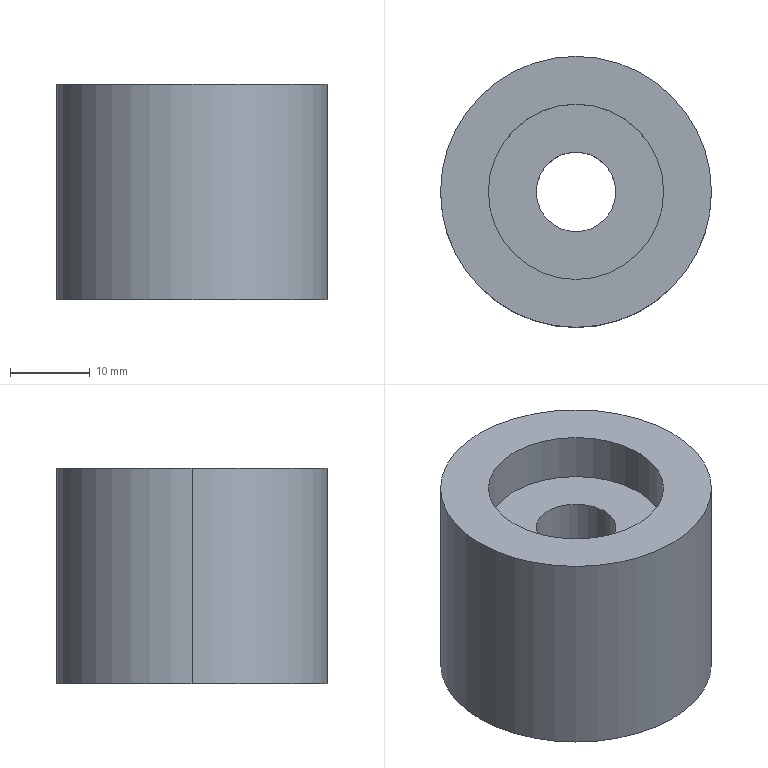Part | STEP file | Driven pulley shaft QY-1-34 | 1 solid | 12 faces | box 34 x 34 x 27 mm | volume 18774 mm3 | cylinder 8 | plane 4 | commonest cylinder face diameters 22 x4 10 x2 34 x2
STEP:
#1=CARTESIAN_POINT('',(0.,0.,0.));
#2=DIRECTION('',(0.,0.,1.));
#3=DIRECTION('',(1.,0.,0.));
#4=AXIS2_PLACEMENT_3D('',#1,#2,#3);
#5=CARTESIAN_POINT('',(-11.,0.,6.));
#6=VERTEX_POINT('',#5);
#7=CARTESIAN_POINT('',(-11.,0.,0.));
#8=VERTEX_POINT('',#7);
#9=CARTESIAN_POINT('',(-11.,0.,6.));
#10=DIRECTION('',(0.,0.,-1.));
#11=VECTOR('',#10,1.);
#12=LINE('',#9,#11);
#13=CARTESIAN_POINT('',(0.,0.,6.));
#14=DIRECTION('',(0.,0.,-1.));
#15=DIRECTION('',(-1.,0.,0.));
#16=AXIS2_PLACEMENT_3D('',#13,#14,#15);
#17=CYLINDRICAL_SURFACE('',#16,11.);
#18=CARTESIAN_POINT('',(6.283,0.));
#19=DIRECTION('',(0.,1.));
#20=VECTOR('',#19,1.);
#21=LINE('',#18,#20);
#22=(GEOMETRIC_REPRESENTATION_CONTEXT(2)PARAMETRIC_REPRESENTATION_CONTEXT()REPRESENTATION_CONTEXT('',''));
#23=DEFINITIONAL_REPRESENTATION('',(#21),#22);
#24=PCURVE('',#17,#23);
#25=CARTESIAN_POINT('',(0.,0.,6.));
#26=DIRECTION('',(0.,0.,-1.));
#27=DIRECTION('',(-1.,0.,0.));
#28=AXIS2_PLACEMENT_3D('',#25,#26,#27);
#29=CYLINDRICAL_SURFACE('',#28,11.);
#30=CARTESIAN_POINT('',(0.,0.));
#31=DIRECTION('',(0.,1.));
#32=VECTOR('',#31,1.);
#33=LINE('',#30,#32);
#34=(GEOMETRIC_REPRESENTATION_CONTEXT(2)PARAMETRIC_REPRESENTATION_CONTEXT()REPRESENTATION_CONTEXT('',''));
#35=DEFINITIONAL_REPRESENTATION('',(#33),#34);
#36=PCURVE('',#29,#35);
#37=SURFACE_CURVE('',#12,(#24,#36),.PCURVE_S1.);
#38=EDGE_CURVE('',#6,#8,#37,.T.);
#39=ORIENTED_EDGE('',*,*,#38,.T.);
#40=CARTESIAN_POINT('',(11.,0.,0.));
#41=VERTEX_POINT('',#40);
#42=CARTESIAN_POINT('',(0.,0.,0.));
#43=DIRECTION('',(0.,0.,-1.));
#44=DIRECTION('',(-1.,0.,0.));
#45=AXIS2_PLACEMENT_3D('',#42,#43,#44);
#46=CIRCLE('',#45,11.);
#47=CARTESIAN_POINT('',(0.,6.));
#48=DIRECTION('',(1.,0.));
#49=VECTOR('',#48,1.);
#50=LINE('',#47,#49);
#51=(GEOMETRIC_REPRESENTATION_CONTEXT(2)PARAMETRIC_REPRESENTATION_CONTEXT()REPRESENTATION_CONTEXT('',''));
#52=DEFINITIONAL_REPRESENTATION('',(#50),#51);
#53=PCURVE('',#17,#52);
#54=CARTESIAN_POINT('',(0.,0.,0.));
#55=DIRECTION('',(0.,0.,1.));
#56=DIRECTION('',(1.,0.,0.));
#57=AXIS2_PLACEMENT_3D('',#54,#55,#56);
#58=PLANE('',#57);
#59=CARTESIAN_POINT('',(-11.,0.));
#60=CARTESIAN_POINT('',(-11.,19.053));
#61=CARTESIAN_POINT('',(5.5,9.526));
#62=CARTESIAN_POINT('',(22.,0.));
#63=CARTESIAN_POINT('',(5.5,-9.526));
#64=CARTESIAN_POINT('',(-11.,-19.053));
#65=CARTESIAN_POINT('',(-11.,0.));
#66=(BOUNDED_CURVE()B_SPLINE_CURVE(2,(#59,#60,#61,#62,#63,#64,#65),.UNSPECIFIED.,.T.,.F.)B_SPLINE_CURVE_WITH_KNOTS((1,2,2,2,2,1),(-2.094,0.,2.094,4.189,6.283,8.378),.UNSPECIFIED.)CURVE()GEOMETRIC_REPRESENTATION_ITEM()RATIONAL_B_SPLINE_CURVE((1.,0.5,1.,0.5,1.,0.5,1.))REPRESENTATION_ITEM(''));
#67=(GEOMETRIC_REPRESENTATION_CONTEXT(2)PARAMETRIC_REPRESENTATION_CONTEXT()REPRESENTATION_CONTEXT('',''));
#68=DEFINITIONAL_REPRESENTATION('',(#66),#67);
#69=PCURVE('',#58,#68);
#70=SURFACE_CURVE('',#46,(#53,#69),.PCURVE_S1.);
#71=EDGE_CURVE('',#41,#8,#70,.T.);
#72=ORIENTED_EDGE('',*,*,#71,.F.);
#73=CARTESIAN_POINT('',(11.,0.,6.));
#74=VERTEX_POINT('',#73);
#75=CARTESIAN_POINT('',(11.,0.,6.));
#76=DIRECTION('',(0.,0.,-1.));
#77=VECTOR('',#76,1.);
#78=LINE('',#75,#77);
#79=CARTESIAN_POINT('',(3.142,0.));
#80=DIRECTION('',(0.,1.));
#81=VECTOR('',#80,1.);
#82=LINE('',#79,#81);
#83=(GEOMETRIC_REPRESENTATION_CONTEXT(2)PARAMETRIC_REPRESENTATION_CONTEXT()REPRESENTATION_CONTEXT('',''));
#84=DEFINITIONAL_REPRESENTATION('',(#82),#83);
#85=PCURVE('',#17,#84);
#86=CARTESIAN_POINT('',(3.142,0.));
#87=DIRECTION('',(0.,1.));
#88=VECTOR('',#87,1.);
#89=LINE('',#86,#88);
#90=(GEOMETRIC_REPRESENTATION_CONTEXT(2)PARAMETRIC_REPRESENTATION_CONTEXT()REPRESENTATION_CONTEXT('',''));
#91=DEFINITIONAL_REPRESENTATION('',(#89),#90);
#92=PCURVE('',#29,#91);
#93=SURFACE_CURVE('',#78,(#85,#92),.PCURVE_S1.);
#94=EDGE_CURVE('',#74,#41,#93,.T.);
#95=ORIENTED_EDGE('',*,*,#94,.F.);
#96=CARTESIAN_POINT('',(0.,0.,6.));
#97=DIRECTION('',(0.,0.,-1.));
#98=DIRECTION('',(-1.,0.,0.));
#99=AXIS2_PLACEMENT_3D('',#96,#97,#98);
#100=CIRCLE('',#99,11.);
#101=CARTESIAN_POINT('',(0.,0.));
#102=DIRECTION('',(1.,0.));
#103=VECTOR('',#102,1.);
#104=LINE('',#101,#103);
#105=(GEOMETRIC_REPRESENTATION_CONTEXT(2)PARAMETRIC_REPRESENTATION_CONTEXT()REPRESENTATION_CONTEXT('',''));
#106=DEFINITIONAL_REPRESENTATION('',(#104),#105);
#107=PCURVE('',#17,#106);
#108=CARTESIAN_POINT('',(0.,0.,6.));
#109=DIRECTION('',(0.,0.,-1.));
#110=DIRECTION('',(-1.,0.,0.));
#111=AXIS2_PLACEMENT_3D('',#108,#109,#110);
#112=PLANE('',#111);
#113=CARTESIAN_POINT('',(0.,0.));
#114=DIRECTION('',(1.,0.));
#115=AXIS2_PLACEMENT_2D('',#113,#114);
#116=CIRCLE('',#115,11.);
#117=(GEOMETRIC_REPRESENTATION_CONTEXT(2)PARAMETRIC_REPRESENTATION_CONTEXT()REPRESENTATION_CONTEXT('',''));
#118=DEFINITIONAL_REPRESENTATION('',(#116),#117);
#119=PCURVE('',#112,#118);
#120=SURFACE_CURVE('',#100,(#107,#119),.PCURVE_S1.);
#121=EDGE_CURVE('',#74,#6,#120,.T.);
#122=ORIENTED_EDGE('',*,*,#121,.T.);
#123=EDGE_LOOP('',(#39,#72,#95,#122));
#124=FACE_BOUND('',#123,.F.);
#125=ADVANCED_FACE('',(#124),#17,.F.);
#126=CARTESIAN_POINT('',(11.,0.,21.));
#127=VERTEX_POINT('',#126);
#128=CARTESIAN_POINT('',(11.,0.,27.));
#129=VERTEX_POINT('',#128);
#130=CARTESIAN_POINT('',(11.,0.,21.));
#131=DIRECTION('',(0.,0.,1.));
#132=VECTOR('',#131,1.);
#133=LINE('',#130,#132);
#134=CARTESIAN_POINT('',(0.,0.,21.));
#135=DIRECTION('',(0.,0.,1.));
#136=DIRECTION('',(1.,0.,0.));
#137=AXIS2_PLACEMENT_3D('',#134,#135,#136);
#138=CYLINDRICAL_SURFACE('',#137,11.);
#139=CARTESIAN_POINT('',(6.283,0.));
#140=DIRECTION('',(0.,1.));
#141=VECTOR('',#140,1.);
#142=LINE('',#139,#141);
#143=(GEOMETRIC_REPRESENTATION_CONTEXT(2)PARAMETRIC_REPRESENTATION_CONTEXT()REPRESENTATION_CONTEXT('',''));
#144=DEFINITIONAL_REPRESENTATION('',(#142),#143);
#145=PCURVE('',#138,#144);
#146=CARTESIAN_POINT('',(0.,0.,21.));
#147=DIRECTION('',(0.,0.,1.));
#148=DIRECTION('',(1.,0.,0.));
#149=AXIS2_PLACEMENT_3D('',#146,#147,#148);
#150=CYLINDRICAL_SURFACE('',#149,11.);
#151=CARTESIAN_POINT('',(0.,0.));
#152=DIRECTION('',(0.,1.));
#153=VECTOR('',#152,1.);
#154=LINE('',#151,#153);
#155=(GEOMETRIC_REPRESENTATION_CONTEXT(2)PARAMETRIC_REPRESENTATION_CONTEXT()REPRESENTATION_CONTEXT('',''));
#156=DEFINITIONAL_REPRESENTATION('',(#154),#155);
#157=PCURVE('',#150,#156);
#158=SURFACE_CURVE('',#133,(#145,#157),.PCURVE_S1.);
#159=EDGE_CURVE('',#127,#129,#158,.T.);
#160=ORIENTED_EDGE('',*,*,#159,.T.);
#161=CARTESIAN_POINT('',(-11.,0.,27.));
#162=VERTEX_POINT('',#161);
#163=CARTESIAN_POINT('',(0.,0.,27.));
#164=DIRECTION('',(0.,0.,1.));
#165=DIRECTION('',(1.,0.,0.));
#166=AXIS2_PLACEMENT_3D('',#163,#164,#165);
#167=CIRCLE('',#166,11.);
#168=CARTESIAN_POINT('',(0.,6.));
#169=DIRECTION('',(1.,0.));
#170=VECTOR('',#169,1.);
#171=LINE('',#168,#170);
#172=(GEOMETRIC_REPRESENTATION_CONTEXT(2)PARAMETRIC_REPRESENTATION_CONTEXT()REPRESENTATION_CONTEXT('',''));
#173=DEFINITIONAL_REPRESENTATION('',(#171),#172);
#174=PCURVE('',#138,#173);
#175=CARTESIAN_POINT('',(0.,0.,27.));
#176=DIRECTION('',(0.,0.,1.));
#177=DIRECTION('',(1.,0.,0.));
#178=AXIS2_PLACEMENT_3D('',#175,#176,#177);
#179=PLANE('',#178);
#180=CARTESIAN_POINT('',(0.,0.));
#181=DIRECTION('',(1.,0.));
#182=AXIS2_PLACEMENT_2D('',#180,#181);
#183=CIRCLE('',#182,11.);
#184=(GEOMETRIC_REPRESENTATION_CONTEXT(2)PARAMETRIC_REPRESENTATION_CONTEXT()REPRESENTATION_CONTEXT('',''));
#185=DEFINITIONAL_REPRESENTATION('',(#183),#184);
#186=PCURVE('',#179,#185);
#187=SURFACE_CURVE('',#167,(#174,#186),.PCURVE_S1.);
#188=EDGE_CURVE('',#162,#129,#187,.T.);
#189=ORIENTED_EDGE('',*,*,#188,.F.);
#190=CARTESIAN_POINT('',(-11.,0.,21.));
#191=VERTEX_POINT('',#190);
#192=CARTESIAN_POINT('',(-11.,0.,21.));
#193=DIRECTION('',(0.,0.,1.));
#194=VECTOR('',#193,1.);
#195=LINE('',#192,#194);
#196=CARTESIAN_POINT('',(3.142,0.));
#197=DIRECTION('',(0.,1.));
#198=VECTOR('',#197,1.);
#199=LINE('',#196,#198);
#200=(GEOMETRIC_REPRESENTATION_CONTEXT(2)PARAMETRIC_REPRESENTATION_CONTEXT()REPRESENTATION_CONTEXT('',''));
#201=DEFINITIONAL_REPRESENTATION('',(#199),#200);
#202=PCURVE('',#138,#201);
#203=CARTESIAN_POINT('',(3.142,0.));
#204=DIRECTION('',(0.,1.));
#205=VECTOR('',#204,1.);
#206=LINE('',#203,#205);
#207=(GEOMETRIC_REPRESENTATION_CONTEXT(2)PARAMETRIC_REPRESENTATION_CONTEXT()REPRESENTATION_CONTEXT('',''));
#208=DEFINITIONAL_REPRESENTATION('',(#206),#207);
#209=PCURVE('',#150,#208);
#210=SURFACE_CURVE('',#195,(#202,#209),.PCURVE_S1.);
#211=EDGE_CURVE('',#191,#162,#210,.T.);
#212=ORIENTED_EDGE('',*,*,#211,.F.);
#213=CARTESIAN_POINT('',(0.,0.,21.));
#214=DIRECTION('',(0.,0.,1.));
#215=DIRECTION('',(1.,0.,0.));
#216=AXIS2_PLACEMENT_3D('',#213,#214,#215);
#217=CIRCLE('',#216,11.);
#218=CARTESIAN_POINT('',(0.,0.));
#219=DIRECTION('',(1.,0.));
#220=VECTOR('',#219,1.);
#221=LINE('',#218,#220);
#222=(GEOMETRIC_REPRESENTATION_CONTEXT(2)PARAMETRIC_REPRESENTATION_CONTEXT()REPRESENTATION_CONTEXT('',''));
#223=DEFINITIONAL_REPRESENTATION('',(#221),#222);
#224=PCURVE('',#138,#223);
#225=CARTESIAN_POINT('',(0.,0.,21.));
#226=DIRECTION('',(0.,0.,1.));
#227=DIRECTION('',(1.,0.,0.));
#228=AXIS2_PLACEMENT_3D('',#225,#226,#227);
#229=PLANE('',#228);
#230=CARTESIAN_POINT('',(0.,0.));
#231=DIRECTION('',(1.,0.));
#232=AXIS2_PLACEMENT_2D('',#230,#231);
#233=CIRCLE('',#232,11.);
#234=(GEOMETRIC_REPRESENTATION_CONTEXT(2)PARAMETRIC_REPRESENTATION_CONTEXT()REPRESENTATION_CONTEXT('',''));
#235=DEFINITIONAL_REPRESENTATION('',(#233),#234);
#236=PCURVE('',#229,#235);
#237=SURFACE_CURVE('',#217,(#224,#236),.PCURVE_S1.);
#238=EDGE_CURVE('',#191,#127,#237,.T.);
#239=ORIENTED_EDGE('',*,*,#238,.T.);
#240=EDGE_LOOP('',(#160,#189,#212,#239));
#241=FACE_BOUND('',#240,.F.);
#242=ADVANCED_FACE('',(#241),#138,.F.);
#243=CARTESIAN_POINT('',(17.,0.,27.));
#244=VERTEX_POINT('',#243);
#245=CARTESIAN_POINT('',(-17.,0.,27.));
#246=VERTEX_POINT('',#245);
#247=CARTESIAN_POINT('',(0.,0.,27.));
#248=DIRECTION('',(0.,0.,1.));
#249=DIRECTION('',(1.,0.,0.));
#250=AXIS2_PLACEMENT_3D('',#247,#248,#249);
#251=CIRCLE('',#250,17.);
#252=CARTESIAN_POINT('',(0.,0.,27.));
#253=DIRECTION('',(0.,0.,-1.));
#254=DIRECTION('',(-1.,0.,0.));
#255=AXIS2_PLACEMENT_3D('',#252,#253,#254);
#256=CYLINDRICAL_SURFACE('',#255,17.);
#257=CARTESIAN_POINT('',(3.142,0.));
#258=DIRECTION('',(-1.,0.));
#259=VECTOR('',#258,1.);
#260=LINE('',#257,#259);
#261=(GEOMETRIC_REPRESENTATION_CONTEXT(2)PARAMETRIC_REPRESENTATION_CONTEXT()REPRESENTATION_CONTEXT('',''));
#262=DEFINITIONAL_REPRESENTATION('',(#260),#261);
#263=PCURVE('',#256,#262);
#264=CARTESIAN_POINT('',(0.,0.));
#265=DIRECTION('',(1.,0.));
#266=AXIS2_PLACEMENT_2D('',#264,#265);
#267=CIRCLE('',#266,17.);
#268=(GEOMETRIC_REPRESENTATION_CONTEXT(2)PARAMETRIC_REPRESENTATION_CONTEXT()REPRESENTATION_CONTEXT('',''));
#269=DEFINITIONAL_REPRESENTATION('',(#267),#268);
#270=PCURVE('',#179,#269);
#271=SURFACE_CURVE('',#251,(#263,#270),.PCURVE_S1.);
#272=EDGE_CURVE('',#244,#246,#271,.T.);
#273=ORIENTED_EDGE('',*,*,#272,.F.);
#274=CARTESIAN_POINT('',(17.,0.,0.));
#275=VERTEX_POINT('',#274);
#276=CARTESIAN_POINT('',(17.,0.,27.));
#277=DIRECTION('',(0.,0.,-1.));
#278=VECTOR('',#277,1.);
#279=LINE('',#276,#278);
#280=CARTESIAN_POINT('',(3.142,0.));
#281=DIRECTION('',(0.,1.));
#282=VECTOR('',#281,1.);
#283=LINE('',#280,#282);
#284=(GEOMETRIC_REPRESENTATION_CONTEXT(2)PARAMETRIC_REPRESENTATION_CONTEXT()REPRESENTATION_CONTEXT('',''));
#285=DEFINITIONAL_REPRESENTATION('',(#283),#284);
#286=PCURVE('',#256,#285);
#287=CARTESIAN_POINT('',(0.,0.,27.));
#288=DIRECTION('',(0.,0.,-1.));
#289=DIRECTION('',(-1.,0.,0.));
#290=AXIS2_PLACEMENT_3D('',#287,#288,#289);
#291=CYLINDRICAL_SURFACE('',#290,17.);
#292=CARTESIAN_POINT('',(3.142,0.));
#293=DIRECTION('',(0.,1.));
#294=VECTOR('',#293,1.);
#295=LINE('',#292,#294);
#296=(GEOMETRIC_REPRESENTATION_CONTEXT(2)PARAMETRIC_REPRESENTATION_CONTEXT()REPRESENTATION_CONTEXT('',''));
#297=DEFINITIONAL_REPRESENTATION('',(#295),#296);
#298=PCURVE('',#291,#297);
#299=SURFACE_CURVE('',#279,(#286,#298),.PCURVE_S1.);
#300=EDGE_CURVE('',#244,#275,#299,.T.);
#301=ORIENTED_EDGE('',*,*,#300,.T.);
#302=CARTESIAN_POINT('',(-17.,0.,0.));
#303=VERTEX_POINT('',#302);
#304=CARTESIAN_POINT('',(0.,0.,0.));
#305=DIRECTION('',(0.,0.,1.));
#306=DIRECTION('',(1.,0.,0.));
#307=AXIS2_PLACEMENT_3D('',#304,#305,#306);
#308=CIRCLE('',#307,17.);
#309=CARTESIAN_POINT('',(3.142,27.));
#310=DIRECTION('',(-1.,0.));
#311=VECTOR('',#310,1.);
#312=LINE('',#309,#311);
#313=(GEOMETRIC_REPRESENTATION_CONTEXT(2)PARAMETRIC_REPRESENTATION_CONTEXT()REPRESENTATION_CONTEXT('',''));
#314=DEFINITIONAL_REPRESENTATION('',(#312),#313);
#315=PCURVE('',#256,#314);
#316=CARTESIAN_POINT('',(0.,0.));
#317=DIRECTION('',(1.,0.));
#318=AXIS2_PLACEMENT_2D('',#316,#317);
#319=CIRCLE('',#318,17.);
#320=(GEOMETRIC_REPRESENTATION_CONTEXT(2)PARAMETRIC_REPRESENTATION_CONTEXT()REPRESENTATION_CONTEXT('',''));
#321=DEFINITIONAL_REPRESENTATION('',(#319),#320);
#322=PCURVE('',#58,#321);
#323=SURFACE_CURVE('',#308,(#315,#322),.PCURVE_S1.);
#324=EDGE_CURVE('',#275,#303,#323,.T.);
#325=ORIENTED_EDGE('',*,*,#324,.T.);
#326=CARTESIAN_POINT('',(-17.,0.,27.));
#327=DIRECTION('',(0.,0.,-1.));
#328=VECTOR('',#327,1.);
#329=LINE('',#326,#328);
#330=CARTESIAN_POINT('',(0.,0.));
#331=DIRECTION('',(0.,1.));
#332=VECTOR('',#331,1.);
#333=LINE('',#330,#332);
#334=(GEOMETRIC_REPRESENTATION_CONTEXT(2)PARAMETRIC_REPRESENTATION_CONTEXT()REPRESENTATION_CONTEXT('',''));
#335=DEFINITIONAL_REPRESENTATION('',(#333),#334);
#336=PCURVE('',#256,#335);
#337=CARTESIAN_POINT('',(6.283,0.));
#338=DIRECTION('',(0.,1.));
#339=VECTOR('',#338,1.);
#340=LINE('',#337,#339);
#341=(GEOMETRIC_REPRESENTATION_CONTEXT(2)PARAMETRIC_REPRESENTATION_CONTEXT()REPRESENTATION_CONTEXT('',''));
#342=DEFINITIONAL_REPRESENTATION('',(#340),#341);
#343=PCURVE('',#291,#342);
#344=SURFACE_CURVE('',#329,(#336,#343),.PCURVE_S1.);
#345=EDGE_CURVE('',#246,#303,#344,.T.);
#346=ORIENTED_EDGE('',*,*,#345,.F.);
#347=EDGE_LOOP('',(#273,#301,#325,#346));
#348=FACE_BOUND('',#347,.T.);
#349=ADVANCED_FACE('',(#348),#256,.T.);
#350=CARTESIAN_POINT('',(5.,0.,6.));
#351=VERTEX_POINT('',#350);
#352=CARTESIAN_POINT('',(5.,0.,21.));
#353=VERTEX_POINT('',#352);
#354=CARTESIAN_POINT('',(5.,0.,-29.));
#355=DIRECTION('',(0.,0.,1.));
#356=VECTOR('',#355,1.);
#357=LINE('',#354,#356);
#358=CARTESIAN_POINT('',(0.,0.,-29.));
#359=DIRECTION('',(0.,0.,1.));
#360=DIRECTION('',(1.,0.,0.));
#361=AXIS2_PLACEMENT_3D('',#358,#359,#360);
#362=CYLINDRICAL_SURFACE('',#361,5.);
#363=CARTESIAN_POINT('',(6.283,0.));
#364=DIRECTION('',(0.,1.));
#365=VECTOR('',#364,1.);
#366=LINE('',#363,#365);
#367=(GEOMETRIC_REPRESENTATION_CONTEXT(2)PARAMETRIC_REPRESENTATION_CONTEXT()REPRESENTATION_CONTEXT('',''));
#368=DEFINITIONAL_REPRESENTATION('',(#366),#367);
#369=PCURVE('',#362,#368);
#370=CARTESIAN_POINT('',(0.,0.,-29.));
#371=DIRECTION('',(0.,0.,1.));
#372=DIRECTION('',(1.,0.,0.));
#373=AXIS2_PLACEMENT_3D('',#370,#371,#372);
#374=CYLINDRICAL_SURFACE('',#373,5.);
#375=CARTESIAN_POINT('',(0.,0.));
#376=DIRECTION('',(0.,1.));
#377=VECTOR('',#376,1.);
#378=LINE('',#375,#377);
#379=(GEOMETRIC_REPRESENTATION_CONTEXT(2)PARAMETRIC_REPRESENTATION_CONTEXT()REPRESENTATION_CONTEXT('',''));
#380=DEFINITIONAL_REPRESENTATION('',(#378),#379);
#381=PCURVE('',#374,#380);
#382=SURFACE_CURVE('',#357,(#369,#381),.PCURVE_S1.);
#383=EDGE_CURVE('',#351,#353,#382,.T.);
#384=ORIENTED_EDGE('',*,*,#383,.T.);
#385=CARTESIAN_POINT('',(-5.,0.,21.));
#386=VERTEX_POINT('',#385);
#387=CARTESIAN_POINT('',(0.,0.,21.));
#388=DIRECTION('',(0.,0.,-1.));
#389=DIRECTION('',(1.,0.,0.));
#390=AXIS2_PLACEMENT_3D('',#387,#388,#389);
#391=CIRCLE('',#390,5.);
#392=CARTESIAN_POINT('',(6.283,50.));
#393=DIRECTION('',(-1.,0.));
#394=VECTOR('',#393,1.);
#395=LINE('',#392,#394);
#396=(GEOMETRIC_REPRESENTATION_CONTEXT(2)PARAMETRIC_REPRESENTATION_CONTEXT()REPRESENTATION_CONTEXT('',''));
#397=DEFINITIONAL_REPRESENTATION('',(#395),#396);
#398=PCURVE('',#362,#397);
#399=CARTESIAN_POINT('',(5.,0.));
#400=CARTESIAN_POINT('',(5.,-8.66));
#401=CARTESIAN_POINT('',(-2.5,-4.33));
#402=CARTESIAN_POINT('',(-10.,0.));
#403=CARTESIAN_POINT('',(-2.5,4.33));
#404=CARTESIAN_POINT('',(5.,8.66));
#405=CARTESIAN_POINT('',(5.,0.));
#406=(BOUNDED_CURVE()B_SPLINE_CURVE(2,(#399,#400,#401,#402,#403,#404,#405),.UNSPECIFIED.,.T.,.F.)B_SPLINE_CURVE_WITH_KNOTS((1,2,2,2,2,1),(-2.094,0.,2.094,4.189,6.283,8.378),.UNSPECIFIED.)CURVE()GEOMETRIC_REPRESENTATION_ITEM()RATIONAL_B_SPLINE_CURVE((1.,0.5,1.,0.5,1.,0.5,1.))REPRESENTATION_ITEM(''));
#407=(GEOMETRIC_REPRESENTATION_CONTEXT(2)PARAMETRIC_REPRESENTATION_CONTEXT()REPRESENTATION_CONTEXT('',''));
#408=DEFINITIONAL_REPRESENTATION('',(#406),#407);
#409=PCURVE('',#229,#408);
#410=SURFACE_CURVE('',#391,(#398,#409),.PCURVE_S1.);
#411=EDGE_CURVE('',#353,#386,#410,.T.);
#412=ORIENTED_EDGE('',*,*,#411,.T.);
#413=CARTESIAN_POINT('',(-5.,0.,6.));
#414=VERTEX_POINT('',#413);
#415=CARTESIAN_POINT('',(-5.,0.,-29.));
#416=DIRECTION('',(0.,0.,1.));
#417=VECTOR('',#416,1.);
#418=LINE('',#415,#417);
#419=CARTESIAN_POINT('',(3.142,0.));
#420=DIRECTION('',(0.,1.));
#421=VECTOR('',#420,1.);
#422=LINE('',#419,#421);
#423=(GEOMETRIC_REPRESENTATION_CONTEXT(2)PARAMETRIC_REPRESENTATION_CONTEXT()REPRESENTATION_CONTEXT('',''));
#424=DEFINITIONAL_REPRESENTATION('',(#422),#423);
#425=PCURVE('',#362,#424);
#426=CARTESIAN_POINT('',(3.142,0.));
#427=DIRECTION('',(0.,1.));
#428=VECTOR('',#427,1.);
#429=LINE('',#426,#428);
#430=(GEOMETRIC_REPRESENTATION_CONTEXT(2)PARAMETRIC_REPRESENTATION_CONTEXT()REPRESENTATION_CONTEXT('',''));
#431=DEFINITIONAL_REPRESENTATION('',(#429),#430);
#432=PCURVE('',#374,#431);
#433=SURFACE_CURVE('',#418,(#425,#432),.PCURVE_S1.);
#434=EDGE_CURVE('',#414,#386,#433,.T.);
#435=ORIENTED_EDGE('',*,*,#434,.F.);
#436=CARTESIAN_POINT('',(0.,0.,6.));
#437=DIRECTION('',(0.,0.,1.));
#438=DIRECTION('',(-1.,0.,0.));
#439=AXIS2_PLACEMENT_3D('',#436,#437,#438);
#440=CIRCLE('',#439,5.);
#441=CARTESIAN_POINT('',(3.142,35.));
#442=DIRECTION('',(1.,0.));
#443=VECTOR('',#442,1.);
#444=LINE('',#441,#443);
#445=(GEOMETRIC_REPRESENTATION_CONTEXT(2)PARAMETRIC_REPRESENTATION_CONTEXT()REPRESENTATION_CONTEXT('',''));
#446=DEFINITIONAL_REPRESENTATION('',(#444),#445);
#447=PCURVE('',#362,#446);
#448=CARTESIAN_POINT('',(5.,0.));
#449=CARTESIAN_POINT('',(5.,-8.66));
#450=CARTESIAN_POINT('',(-2.5,-4.33));
#451=CARTESIAN_POINT('',(-10.,0.));
#452=CARTESIAN_POINT('',(-2.5,4.33));
#453=CARTESIAN_POINT('',(5.,8.66));
#454=CARTESIAN_POINT('',(5.,0.));
#455=(BOUNDED_CURVE()B_SPLINE_CURVE(2,(#448,#449,#450,#451,#452,#453,#454),.UNSPECIFIED.,.T.,.F.)B_SPLINE_CURVE_WITH_KNOTS((1,2,2,2,2,1),(-2.094,0.,2.094,4.189,6.283,8.378),.UNSPECIFIED.)CURVE()GEOMETRIC_REPRESENTATION_ITEM()RATIONAL_B_SPLINE_CURVE((1.,0.5,1.,0.5,1.,0.5,1.))REPRESENTATION_ITEM(''));
#456=(GEOMETRIC_REPRESENTATION_CONTEXT(2)PARAMETRIC_REPRESENTATION_CONTEXT()REPRESENTATION_CONTEXT('',''));
#457=DEFINITIONAL_REPRESENTATION('',(#455),#456);
#458=PCURVE('',#112,#457);
#459=SURFACE_CURVE('',#440,(#447,#458),.PCURVE_S1.);
#460=EDGE_CURVE('',#414,#351,#459,.T.);
#461=ORIENTED_EDGE('',*,*,#460,.T.);
#462=EDGE_LOOP('',(#384,#412,#435,#461));
#463=FACE_BOUND('',#462,.F.);
#464=ADVANCED_FACE('',(#463),#362,.F.);
#465=CARTESIAN_POINT('',(0.,0.,21.));
#466=DIRECTION('',(0.,0.,-1.));
#467=DIRECTION('',(1.,0.,0.));
#468=AXIS2_PLACEMENT_3D('',#465,#466,#467);
#469=CIRCLE('',#468,5.);
#470=CARTESIAN_POINT('',(6.283,50.));
#471=DIRECTION('',(-1.,0.));
#472=VECTOR('',#471,1.);
#473=LINE('',#470,#472);
#474=(GEOMETRIC_REPRESENTATION_CONTEXT(2)PARAMETRIC_REPRESENTATION_CONTEXT()REPRESENTATION_CONTEXT('',''));
#475=DEFINITIONAL_REPRESENTATION('',(#473),#474);
#476=PCURVE('',#374,#475);
#477=CARTESIAN_POINT('',(5.,0.));
#478=CARTESIAN_POINT('',(5.,-8.66));
#479=CARTESIAN_POINT('',(-2.5,-4.33));
#480=CARTESIAN_POINT('',(-10.,0.));
#481=CARTESIAN_POINT('',(-2.5,4.33));
#482=CARTESIAN_POINT('',(5.,8.66));
#483=CARTESIAN_POINT('',(5.,0.));
#484=(BOUNDED_CURVE()B_SPLINE_CURVE(2,(#477,#478,#479,#480,#481,#482,#483),.UNSPECIFIED.,.T.,.F.)B_SPLINE_CURVE_WITH_KNOTS((1,2,2,2,2,1),(-2.094,0.,2.094,4.189,6.283,8.378),.UNSPECIFIED.)CURVE()GEOMETRIC_REPRESENTATION_ITEM()RATIONAL_B_SPLINE_CURVE((1.,0.5,1.,0.5,1.,0.5,1.))REPRESENTATION_ITEM(''));
#485=(GEOMETRIC_REPRESENTATION_CONTEXT(2)PARAMETRIC_REPRESENTATION_CONTEXT()REPRESENTATION_CONTEXT('',''));
#486=DEFINITIONAL_REPRESENTATION('',(#484),#485);
#487=PCURVE('',#229,#486);
#488=SURFACE_CURVE('',#469,(#476,#487),.PCURVE_S1.);
#489=EDGE_CURVE('',#386,#353,#488,.T.);
#490=ORIENTED_EDGE('',*,*,#489,.T.);
#491=ORIENTED_EDGE('',*,*,#383,.F.);
#492=CARTESIAN_POINT('',(0.,0.,6.));
#493=DIRECTION('',(0.,0.,1.));
#494=DIRECTION('',(-1.,0.,0.));
#495=AXIS2_PLACEMENT_3D('',#492,#493,#494);
#496=CIRCLE('',#495,5.);
#497=CARTESIAN_POINT('',(-3.142,35.));
#498=DIRECTION('',(1.,0.));
#499=VECTOR('',#498,1.);
#500=LINE('',#497,#499);
#501=(GEOMETRIC_REPRESENTATION_CONTEXT(2)PARAMETRIC_REPRESENTATION_CONTEXT()REPRESENTATION_CONTEXT('',''));
#502=DEFINITIONAL_REPRESENTATION('',(#500),#501);
#503=PCURVE('',#374,#502);
#504=CARTESIAN_POINT('',(5.,0.));
#505=CARTESIAN_POINT('',(5.,-8.66));
#506=CARTESIAN_POINT('',(-2.5,-4.33));
#507=CARTESIAN_POINT('',(-10.,0.));
#508=CARTESIAN_POINT('',(-2.5,4.33));
#509=CARTESIAN_POINT('',(5.,8.66));
#510=CARTESIAN_POINT('',(5.,0.));
#511=(BOUNDED_CURVE()B_SPLINE_CURVE(2,(#504,#505,#506,#507,#508,#509,#510),.UNSPECIFIED.,.T.,.F.)B_SPLINE_CURVE_WITH_KNOTS((1,2,2,2,2,1),(-2.094,0.,2.094,4.189,6.283,8.378),.UNSPECIFIED.)CURVE()GEOMETRIC_REPRESENTATION_ITEM()RATIONAL_B_SPLINE_CURVE((1.,0.5,1.,0.5,1.,0.5,1.))REPRESENTATION_ITEM(''));
#512=(GEOMETRIC_REPRESENTATION_CONTEXT(2)PARAMETRIC_REPRESENTATION_CONTEXT()REPRESENTATION_CONTEXT('',''));
#513=DEFINITIONAL_REPRESENTATION('',(#511),#512);
#514=PCURVE('',#112,#513);
#515=SURFACE_CURVE('',#496,(#503,#514),.PCURVE_S1.);
#516=EDGE_CURVE('',#351,#414,#515,.T.);
#517=ORIENTED_EDGE('',*,*,#516,.T.);
#518=ORIENTED_EDGE('',*,*,#434,.T.);
#519=EDGE_LOOP('',(#490,#491,#517,#518));
#520=FACE_BOUND('',#519,.F.);
#521=ADVANCED_FACE('',(#520),#374,.F.);
#522=ORIENTED_EDGE('',*,*,#300,.F.);
#523=CARTESIAN_POINT('',(0.,0.,27.));
#524=DIRECTION('',(0.,0.,1.));
#525=DIRECTION('',(1.,0.,0.));
#526=AXIS2_PLACEMENT_3D('',#523,#524,#525);
#527=CIRCLE('',#526,17.);
#528=CARTESIAN_POINT('',(9.425,0.));
#529=DIRECTION('',(-1.,0.));
#530=VECTOR('',#529,1.);
#531=LINE('',#528,#530);
#532=(GEOMETRIC_REPRESENTATION_CONTEXT(2)PARAMETRIC_REPRESENTATION_CONTEXT()REPRESENTATION_CONTEXT('',''));
#533=DEFINITIONAL_REPRESENTATION('',(#531),#532);
#534=PCURVE('',#291,#533);
#535=CARTESIAN_POINT('',(0.,0.));
#536=DIRECTION('',(1.,0.));
#537=AXIS2_PLACEMENT_2D('',#535,#536);
#538=CIRCLE('',#537,17.);
#539=(GEOMETRIC_REPRESENTATION_CONTEXT(2)PARAMETRIC_REPRESENTATION_CONTEXT()REPRESENTATION_CONTEXT('',''));
#540=DEFINITIONAL_REPRESENTATION('',(#538),#539);
#541=PCURVE('',#179,#540);
#542=SURFACE_CURVE('',#527,(#534,#541),.PCURVE_S1.);
#543=EDGE_CURVE('',#246,#244,#542,.T.);
#544=ORIENTED_EDGE('',*,*,#543,.F.);
#545=ORIENTED_EDGE('',*,*,#345,.T.);
#546=CARTESIAN_POINT('',(0.,0.,0.));
#547=DIRECTION('',(0.,0.,1.));
#548=DIRECTION('',(1.,0.,0.));
#549=AXIS2_PLACEMENT_3D('',#546,#547,#548);
#550=CIRCLE('',#549,17.);
#551=CARTESIAN_POINT('',(9.425,27.));
#552=DIRECTION('',(-1.,0.));
#553=VECTOR('',#552,1.);
#554=LINE('',#551,#553);
#555=(GEOMETRIC_REPRESENTATION_CONTEXT(2)PARAMETRIC_REPRESENTATION_CONTEXT()REPRESENTATION_CONTEXT('',''));
#556=DEFINITIONAL_REPRESENTATION('',(#554),#555);
#557=PCURVE('',#291,#556);
#558=CARTESIAN_POINT('',(0.,0.));
#559=DIRECTION('',(1.,0.));
#560=AXIS2_PLACEMENT_2D('',#558,#559);
#561=CIRCLE('',#560,17.);
#562=(GEOMETRIC_REPRESENTATION_CONTEXT(2)PARAMETRIC_REPRESENTATION_CONTEXT()REPRESENTATION_CONTEXT('',''));
#563=DEFINITIONAL_REPRESENTATION('',(#561),#562);
#564=PCURVE('',#58,#563);
#565=SURFACE_CURVE('',#550,(#557,#564),.PCURVE_S1.);
#566=EDGE_CURVE('',#303,#275,#565,.T.);
#567=ORIENTED_EDGE('',*,*,#566,.T.);
#568=EDGE_LOOP('',(#522,#544,#545,#567));
#569=FACE_BOUND('',#568,.T.);
#570=ADVANCED_FACE('',(#569),#291,.T.);
#571=CARTESIAN_POINT('',(0.,0.,27.));
#572=DIRECTION('',(0.,0.,1.));
#573=DIRECTION('',(1.,0.,0.));
#574=AXIS2_PLACEMENT_3D('',#571,#572,#573);
#575=CIRCLE('',#574,11.);
#576=CARTESIAN_POINT('',(0.,0.));
#577=DIRECTION('',(1.,0.));
#578=AXIS2_PLACEMENT_2D('',#576,#577);
#579=CIRCLE('',#578,11.);
#580=(GEOMETRIC_REPRESENTATION_CONTEXT(2)PARAMETRIC_REPRESENTATION_CONTEXT()REPRESENTATION_CONTEXT('',''));
#581=DEFINITIONAL_REPRESENTATION('',(#579),#580);
#582=PCURVE('',#179,#581);
#583=CARTESIAN_POINT('',(0.,6.));
#584=DIRECTION('',(1.,0.));
#585=VECTOR('',#584,1.);
#586=LINE('',#583,#585);
#587=(GEOMETRIC_REPRESENTATION_CONTEXT(2)PARAMETRIC_REPRESENTATION_CONTEXT()REPRESENTATION_CONTEXT('',''));
#588=DEFINITIONAL_REPRESENTATION('',(#586),#587);
#589=PCURVE('',#150,#588);
#590=SURFACE_CURVE('',#575,(#582,#589),.PCURVE_S1.);
#591=EDGE_CURVE('',#129,#162,#590,.T.);
#592=ORIENTED_EDGE('',*,*,#591,.F.);
#593=ORIENTED_EDGE('',*,*,#188,.F.);
#594=EDGE_LOOP('',(#592,#593));
#595=FACE_BOUND('',#594,.T.);
#596=ORIENTED_EDGE('',*,*,#543,.T.);
#597=ORIENTED_EDGE('',*,*,#272,.T.);
#598=EDGE_LOOP('',(#596,#597));
#599=FACE_BOUND('',#598,.T.);
#600=ADVANCED_FACE('',(#595,#599),#179,.T.);
#601=CARTESIAN_POINT('',(0.,0.,0.));
#602=DIRECTION('',(0.,0.,-1.));
#603=DIRECTION('',(-1.,0.,0.));
#604=AXIS2_PLACEMENT_3D('',#601,#602,#603);
#605=CIRCLE('',#604,11.);
#606=CARTESIAN_POINT('',(-11.,0.));
#607=CARTESIAN_POINT('',(-11.,19.053));
#608=CARTESIAN_POINT('',(5.5,9.526));
#609=CARTESIAN_POINT('',(22.,0.));
#610=CARTESIAN_POINT('',(5.5,-9.526));
#611=CARTESIAN_POINT('',(-11.,-19.053));
#612=CARTESIAN_POINT('',(-11.,0.));
#613=(BOUNDED_CURVE()B_SPLINE_CURVE(2,(#606,#607,#608,#609,#610,#611,#612),.UNSPECIFIED.,.T.,.F.)B_SPLINE_CURVE_WITH_KNOTS((1,2,2,2,2,1),(-2.094,0.,2.094,4.189,6.283,8.378),.UNSPECIFIED.)CURVE()GEOMETRIC_REPRESENTATION_ITEM()RATIONAL_B_SPLINE_CURVE((1.,0.5,1.,0.5,1.,0.5,1.))REPRESENTATION_ITEM(''));
#614=(GEOMETRIC_REPRESENTATION_CONTEXT(2)PARAMETRIC_REPRESENTATION_CONTEXT()REPRESENTATION_CONTEXT('',''));
#615=DEFINITIONAL_REPRESENTATION('',(#613),#614);
#616=PCURVE('',#58,#615);
#617=CARTESIAN_POINT('',(0.,6.));
#618=DIRECTION('',(1.,0.));
#619=VECTOR('',#618,1.);
#620=LINE('',#617,#619);
#621=(GEOMETRIC_REPRESENTATION_CONTEXT(2)PARAMETRIC_REPRESENTATION_CONTEXT()REPRESENTATION_CONTEXT('',''));
#622=DEFINITIONAL_REPRESENTATION('',(#620),#621);
#623=PCURVE('',#29,#622);
#624=SURFACE_CURVE('',#605,(#616,#623),.PCURVE_S1.);
#625=EDGE_CURVE('',#8,#41,#624,.T.);
#626=ORIENTED_EDGE('',*,*,#625,.F.);
#627=ORIENTED_EDGE('',*,*,#71,.F.);
#628=EDGE_LOOP('',(#626,#627));
#629=FACE_BOUND('',#628,.T.);
#630=ORIENTED_EDGE('',*,*,#566,.F.);
#631=ORIENTED_EDGE('',*,*,#324,.F.);
#632=EDGE_LOOP('',(#630,#631));
#633=FACE_BOUND('',#632,.T.);
#634=ADVANCED_FACE('',(#629,#633),#58,.F.);
#635=CARTESIAN_POINT('',(0.,0.,21.));
#636=DIRECTION('',(0.,0.,1.));
#637=DIRECTION('',(1.,0.,0.));
#638=AXIS2_PLACEMENT_3D('',#635,#636,#637);
#639=CIRCLE('',#638,11.);
#640=CARTESIAN_POINT('',(0.,0.));
#641=DIRECTION('',(1.,0.));
#642=AXIS2_PLACEMENT_2D('',#640,#641);
#643=CIRCLE('',#642,11.);
#644=(GEOMETRIC_REPRESENTATION_CONTEXT(2)PARAMETRIC_REPRESENTATION_CONTEXT()REPRESENTATION_CONTEXT('',''));
#645=DEFINITIONAL_REPRESENTATION('',(#643),#644);
#646=PCURVE('',#229,#645);
#647=CARTESIAN_POINT('',(0.,0.));
#648=DIRECTION('',(1.,0.));
#649=VECTOR('',#648,1.);
#650=LINE('',#647,#649);
#651=(GEOMETRIC_REPRESENTATION_CONTEXT(2)PARAMETRIC_REPRESENTATION_CONTEXT()REPRESENTATION_CONTEXT('',''));
#652=DEFINITIONAL_REPRESENTATION('',(#650),#651);
#653=PCURVE('',#150,#652);
#654=SURFACE_CURVE('',#639,(#646,#653),.PCURVE_S1.);
#655=EDGE_CURVE('',#127,#191,#654,.T.);
#656=ORIENTED_EDGE('',*,*,#655,.T.);
#657=ORIENTED_EDGE('',*,*,#238,.T.);
#658=EDGE_LOOP('',(#656,#657));
#659=FACE_BOUND('',#658,.T.);
#660=ORIENTED_EDGE('',*,*,#411,.T.);
#661=ORIENTED_EDGE('',*,*,#489,.T.);
#662=EDGE_LOOP('',(#660,#661));
#663=FACE_BOUND('',#662,.T.);
#664=ADVANCED_FACE('',(#659,#663),#229,.T.);
#665=ORIENTED_EDGE('',*,*,#591,.F.);
#666=ORIENTED_EDGE('',*,*,#159,.F.);
#667=ORIENTED_EDGE('',*,*,#655,.T.);
#668=ORIENTED_EDGE('',*,*,#211,.T.);
#669=EDGE_LOOP('',(#665,#666,#667,#668));
#670=FACE_BOUND('',#669,.F.);
#671=ADVANCED_FACE('',(#670),#150,.F.);
#672=CARTESIAN_POINT('',(0.,0.,6.));
#673=DIRECTION('',(0.,0.,-1.));
#674=DIRECTION('',(-1.,0.,0.));
#675=AXIS2_PLACEMENT_3D('',#672,#673,#674);
#676=CIRCLE('',#675,11.);
#677=CARTESIAN_POINT('',(0.,0.));
#678=DIRECTION('',(1.,0.));
#679=AXIS2_PLACEMENT_2D('',#677,#678);
#680=CIRCLE('',#679,11.);
#681=(GEOMETRIC_REPRESENTATION_CONTEXT(2)PARAMETRIC_REPRESENTATION_CONTEXT()REPRESENTATION_CONTEXT('',''));
#682=DEFINITIONAL_REPRESENTATION('',(#680),#681);
#683=PCURVE('',#112,#682);
#684=CARTESIAN_POINT('',(0.,0.));
#685=DIRECTION('',(1.,0.));
#686=VECTOR('',#685,1.);
#687=LINE('',#684,#686);
#688=(GEOMETRIC_REPRESENTATION_CONTEXT(2)PARAMETRIC_REPRESENTATION_CONTEXT()REPRESENTATION_CONTEXT('',''));
#689=DEFINITIONAL_REPRESENTATION('',(#687),#688);
#690=PCURVE('',#29,#689);
#691=SURFACE_CURVE('',#676,(#683,#690),.PCURVE_S1.);
#692=EDGE_CURVE('',#6,#74,#691,.T.);
#693=ORIENTED_EDGE('',*,*,#692,.T.);
#694=ORIENTED_EDGE('',*,*,#121,.T.);
#695=EDGE_LOOP('',(#693,#694));
#696=FACE_BOUND('',#695,.T.);
#697=ORIENTED_EDGE('',*,*,#516,.T.);
#698=ORIENTED_EDGE('',*,*,#460,.T.);
#699=EDGE_LOOP('',(#697,#698));
#700=FACE_BOUND('',#699,.T.);
#701=ADVANCED_FACE('',(#696,#700),#112,.T.);
#702=ORIENTED_EDGE('',*,*,#625,.F.);
#703=ORIENTED_EDGE('',*,*,#38,.F.);
#704=ORIENTED_EDGE('',*,*,#692,.T.);
#705=ORIENTED_EDGE('',*,*,#94,.T.);
#706=EDGE_LOOP('',(#702,#703,#704,#705));
#707=FACE_BOUND('',#706,.F.);
#708=ADVANCED_FACE('',(#707),#29,.F.);
#709=CLOSED_SHELL('',(#125,#242,#349,#464,#521,#570,#600,#634,#664,#671,#701,#708));
#710=MANIFOLD_SOLID_BREP('',#709);
#711=(LENGTH_UNIT()NAMED_UNIT(*)SI_UNIT(.MILLI.,.METRE.));
#712=UNCERTAINTY_MEASURE_WITH_UNIT(LENGTH_MEASURE(0.0000001),#711,'','');
#713=(NAMED_UNIT(*)PLANE_ANGLE_UNIT()SI_UNIT($,.RADIAN.));
#714=(NAMED_UNIT(*)SI_UNIT($,.STERADIAN.)SOLID_ANGLE_UNIT());
#715=(GEOMETRIC_REPRESENTATION_CONTEXT(3)GLOBAL_UNCERTAINTY_ASSIGNED_CONTEXT((#712))GLOBAL_UNIT_ASSIGNED_CONTEXT((#711,#713,#714))REPRESENTATION_CONTEXT('',''));
#716=ADVANCED_BREP_SHAPE_REPRESENTATION('',(#4,#710),#715);